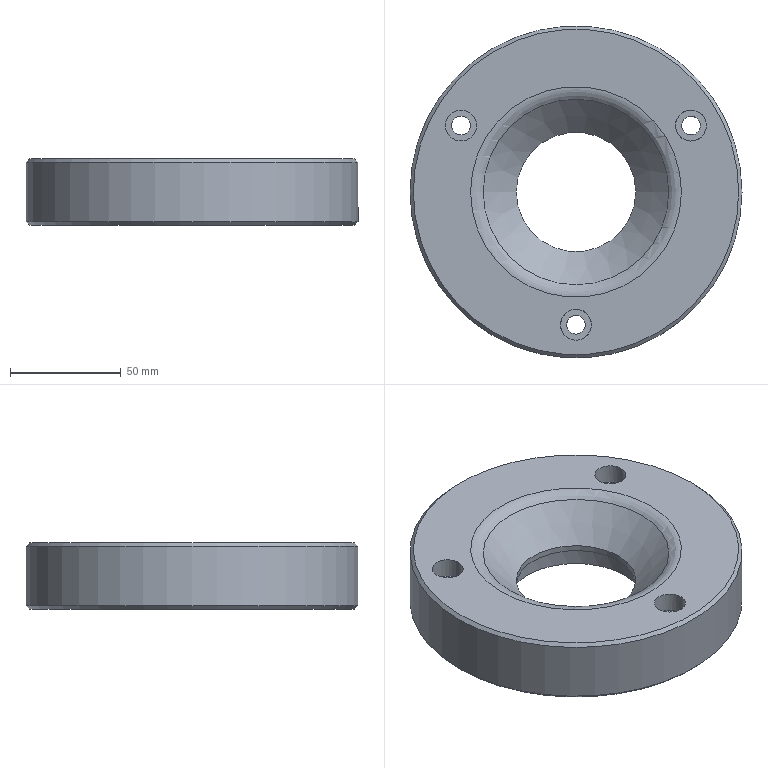Part | STEP file | solid 161 | 1 solid | 19 faces | box 150 x 150 x 30 mm | volume 414170 mm3 | cylinder 9 | plane 6 | cone 3 | torus 1 | commonest cylinder face diameters 8.5 x3 14 x3 54 x1 62 x1 150 x1